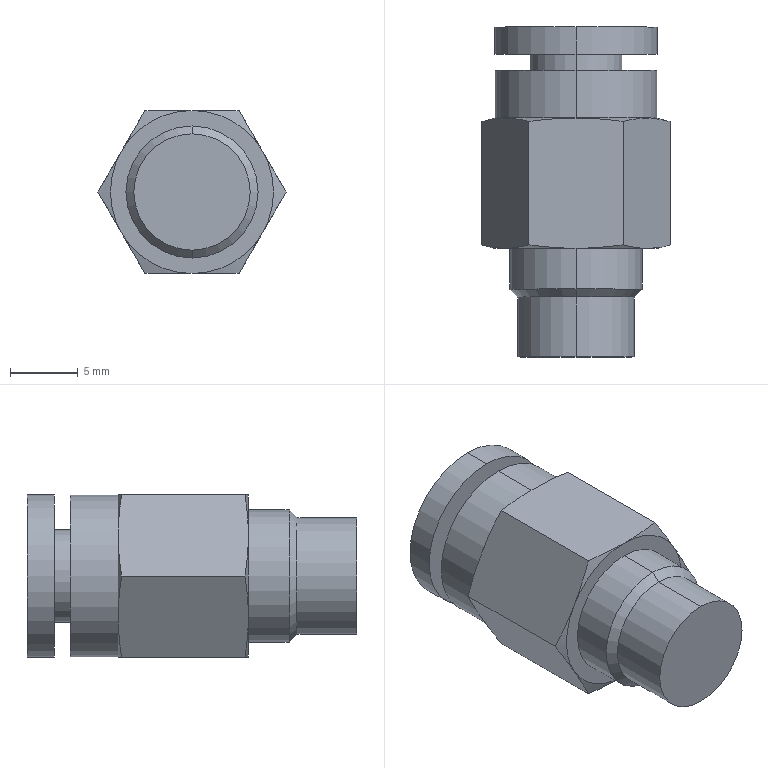Part | STEP file | KQG2H06-01S | 1 solid | 34 faces | box 13.856 x 24.3 x 12 mm | volume 1839 mm3 | cylinder 12 | plane 12 | cone 10 | commonest cylinder face diameters 6 x2 6.8 x2 8.566 x2 9.728 x2 11.9 x2 12 x2
STEP:
#1=CARTESIAN_POINT('',(0.,0.419,4.283));
#2=VERTEX_POINT('',#1);
#3=CARTESIAN_POINT('',(0.,0.419,-4.283));
#4=VERTEX_POINT('',#3);
#5=CARTESIAN_POINT('',(0.,0.419,0.));
#6=DIRECTION('',(0.,-1.,0.));
#7=DIRECTION('',(0.,0.,1.));
#8=AXIS2_PLACEMENT_3D('',#5,#6,#7);
#9=CIRCLE('',#8,4.283);
#10=EDGE_CURVE('',#2,#4,#9,.T.);
#11=ORIENTED_EDGE('',*,*,#10,.F.);
#12=CARTESIAN_POINT('',(0.,1.,4.864));
#13=VERTEX_POINT('',#12);
#14=CARTESIAN_POINT('',(0.,1.,4.864));
#15=DIRECTION('',(0.,0.7071,0.7071));
#16=VECTOR('',#15,1000.);
#17=LINE('',#14,#16);
#18=EDGE_CURVE('',#2,#13,#17,.T.);
#19=ORIENTED_EDGE('',*,*,#18,.T.);
#20=CARTESIAN_POINT('',(0.,1.,-4.864));
#21=VERTEX_POINT('',#20);
#22=CARTESIAN_POINT('',(0.,1.,0.));
#23=DIRECTION('',(0.,-1.,0.));
#24=DIRECTION('',(0.,0.,1.));
#25=AXIS2_PLACEMENT_3D('',#22,#23,#24);
#26=CIRCLE('',#25,4.864);
#27=EDGE_CURVE('',#13,#21,#26,.T.);
#28=ORIENTED_EDGE('',*,*,#27,.T.);
#29=CARTESIAN_POINT('',(0.,1.,-4.864));
#30=DIRECTION('',(0.,0.7071,-0.7071));
#31=VECTOR('',#30,1000.);
#32=LINE('',#29,#31);
#33=EDGE_CURVE('',#4,#21,#32,.T.);
#34=ORIENTED_EDGE('',*,*,#33,.F.);
#35=EDGE_LOOP('',(#11,#19,#28,#34));
#36=FACE_OUTER_BOUND('',#35,.T.);
#37=CARTESIAN_POINT('',(0.,1.,0.));
#38=DIRECTION('',(0.,1.,0.));
#39=DIRECTION('',(0.,0.,-1.));
#40=AXIS2_PLACEMENT_3D('',#37,#38,#39);
#41=CONICAL_SURFACE('',#40,4.864,0.7854);
#42=ADVANCED_FACE('',(#36),#41,.T.);
#43=ORIENTED_EDGE('',*,*,#10,.T.);
#44=CARTESIAN_POINT('',(0.,-4.,-4.283));
#45=VERTEX_POINT('',#44);
#46=CARTESIAN_POINT('',(0.,-5.2,-4.283));
#47=DIRECTION('',(0.,-1.,0.));
#48=VECTOR('',#47,1000.);
#49=LINE('',#46,#48);
#50=EDGE_CURVE('',#4,#45,#49,.T.);
#51=ORIENTED_EDGE('',*,*,#50,.T.);
#52=CARTESIAN_POINT('',(0.,-4.,4.283));
#53=VERTEX_POINT('',#52);
#54=CARTESIAN_POINT('',(0.,-4.,0.));
#55=DIRECTION('',(0.,1.,0.));
#56=DIRECTION('',(0.,0.,1.));
#57=AXIS2_PLACEMENT_3D('',#54,#55,#56);
#58=CIRCLE('',#57,4.283);
#59=EDGE_CURVE('',#45,#53,#58,.T.);
#60=ORIENTED_EDGE('',*,*,#59,.T.);
#61=CARTESIAN_POINT('',(0.,-5.2,4.283));
#62=DIRECTION('',(0.,-1.,0.));
#63=VECTOR('',#62,1000.);
#64=LINE('',#61,#63);
#65=EDGE_CURVE('',#2,#53,#64,.T.);
#66=ORIENTED_EDGE('',*,*,#65,.F.);
#67=EDGE_LOOP('',(#43,#51,#60,#66));
#68=FACE_OUTER_BOUND('',#67,.T.);
#69=CARTESIAN_POINT('',(0.,-5.2,0.));
#70=DIRECTION('',(0.,-1.,0.));
#71=DIRECTION('',(0.,0.,1.));
#72=AXIS2_PLACEMENT_3D('',#69,#70,#71);
#73=CYLINDRICAL_SURFACE('',#72,4.283);
#74=ADVANCED_FACE('',(#68),#73,.T.);
#75=CARTESIAN_POINT('',(0.,1.,0.));
#76=DIRECTION('',(0.,-1.,0.));
#77=DIRECTION('',(0.,0.,1.));
#78=AXIS2_PLACEMENT_3D('',#75,#76,#77);
#79=CIRCLE('',#78,4.864);
#80=EDGE_CURVE('',#21,#13,#79,.T.);
#81=ORIENTED_EDGE('',*,*,#80,.F.);
#82=CARTESIAN_POINT('',(0.,4.,-4.864));
#83=VERTEX_POINT('',#82);
#84=CARTESIAN_POINT('',(0.,20.3,-4.864));
#85=DIRECTION('',(0.,1.,0.));
#86=VECTOR('',#85,1000.);
#87=LINE('',#84,#86);
#88=EDGE_CURVE('',#21,#83,#87,.T.);
#89=ORIENTED_EDGE('',*,*,#88,.T.);
#90=CARTESIAN_POINT('',(0.,4.,4.864));
#91=VERTEX_POINT('',#90);
#92=CARTESIAN_POINT('',(0.,4.,0.));
#93=DIRECTION('',(0.,1.,0.));
#94=DIRECTION('',(0.,0.,1.));
#95=AXIS2_PLACEMENT_3D('',#92,#93,#94);
#96=CIRCLE('',#95,4.864);
#97=EDGE_CURVE('',#91,#83,#96,.T.);
#98=ORIENTED_EDGE('',*,*,#97,.F.);
#99=CARTESIAN_POINT('',(0.,20.3,4.864));
#100=DIRECTION('',(0.,1.,0.));
#101=VECTOR('',#100,1000.);
#102=LINE('',#99,#101);
#103=EDGE_CURVE('',#13,#91,#102,.T.);
#104=ORIENTED_EDGE('',*,*,#103,.F.);
#105=EDGE_LOOP('',(#81,#89,#98,#104));
#106=FACE_OUTER_BOUND('',#105,.T.);
#107=CARTESIAN_POINT('',(0.,20.3,0.));
#108=DIRECTION('',(0.,1.,0.));
#109=DIRECTION('',(0.,0.,1.));
#110=AXIS2_PLACEMENT_3D('',#107,#108,#109);
#111=CYLINDRICAL_SURFACE('',#110,4.864);
#112=ADVANCED_FACE('',(#106),#111,.T.);
#113=CARTESIAN_POINT('',(0.,1.5,-3.));
#114=VERTEX_POINT('',#113);
#115=CARTESIAN_POINT('',(0.,1.5,3.));
#116=VERTEX_POINT('',#115);
#117=CARTESIAN_POINT('',(0.,1.5,0.));
#118=DIRECTION('',(0.,1.,0.));
#119=DIRECTION('',(0.,0.,1.));
#120=AXIS2_PLACEMENT_3D('',#117,#118,#119);
#121=CIRCLE('',#120,3.);
#122=EDGE_CURVE('',#114,#116,#121,.T.);
#123=ORIENTED_EDGE('',*,*,#122,.F.);
#124=CARTESIAN_POINT('',(0.,20.3,-3.));
#125=VERTEX_POINT('',#124);
#126=CARTESIAN_POINT('',(0.,20.3,-3.));
#127=DIRECTION('',(0.,1.,0.));
#128=VECTOR('',#127,1000.);
#129=LINE('',#126,#128);
#130=EDGE_CURVE('',#114,#125,#129,.T.);
#131=ORIENTED_EDGE('',*,*,#130,.T.);
#132=CARTESIAN_POINT('',(0.,20.3,3.));
#133=VERTEX_POINT('',#132);
#134=CARTESIAN_POINT('',(0.,20.3,0.));
#135=DIRECTION('',(0.,1.,0.));
#136=DIRECTION('',(0.,0.,1.));
#137=AXIS2_PLACEMENT_3D('',#134,#135,#136);
#138=CIRCLE('',#137,3.);
#139=EDGE_CURVE('',#125,#133,#138,.T.);
#140=ORIENTED_EDGE('',*,*,#139,.T.);
#141=CARTESIAN_POINT('',(0.,20.3,3.));
#142=DIRECTION('',(0.,1.,0.));
#143=VECTOR('',#142,1000.);
#144=LINE('',#141,#143);
#145=EDGE_CURVE('',#116,#133,#144,.T.);
#146=ORIENTED_EDGE('',*,*,#145,.F.);
#147=EDGE_LOOP('',(#123,#131,#140,#146));
#148=FACE_OUTER_BOUND('',#147,.T.);
#149=CARTESIAN_POINT('',(0.,20.3,0.));
#150=DIRECTION('',(0.,1.,0.));
#151=DIRECTION('',(0.,0.,1.));
#152=AXIS2_PLACEMENT_3D('',#149,#150,#151);
#153=CYLINDRICAL_SURFACE('',#152,3.);
#154=ADVANCED_FACE('',(#148),#153,.F.);
#155=CARTESIAN_POINT('',(0.,18.3,6.));
#156=VERTEX_POINT('',#155);
#157=CARTESIAN_POINT('',(0.,18.3,-6.));
#158=VERTEX_POINT('',#157);
#159=CARTESIAN_POINT('',(0.,18.3,0.));
#160=DIRECTION('',(0.,1.,0.));
#161=DIRECTION('',(0.,0.,1.));
#162=AXIS2_PLACEMENT_3D('',#159,#160,#161);
#163=CIRCLE('',#162,6.);
#164=EDGE_CURVE('',#156,#158,#163,.T.);
#165=ORIENTED_EDGE('',*,*,#164,.T.);
#166=CARTESIAN_POINT('',(0.,20.3,-6.));
#167=VERTEX_POINT('',#166);
#168=CARTESIAN_POINT('',(0.,20.3,-6.));
#169=DIRECTION('',(0.,1.,0.));
#170=VECTOR('',#169,1000.);
#171=LINE('',#168,#170);
#172=EDGE_CURVE('',#158,#167,#171,.T.);
#173=ORIENTED_EDGE('',*,*,#172,.T.);
#174=CARTESIAN_POINT('',(0.,20.3,6.));
#175=VERTEX_POINT('',#174);
#176=CARTESIAN_POINT('',(0.,20.3,0.));
#177=DIRECTION('',(0.,1.,0.));
#178=DIRECTION('',(0.,0.,1.));
#179=AXIS2_PLACEMENT_3D('',#176,#177,#178);
#180=CIRCLE('',#179,6.);
#181=EDGE_CURVE('',#175,#167,#180,.T.);
#182=ORIENTED_EDGE('',*,*,#181,.F.);
#183=CARTESIAN_POINT('',(0.,20.3,6.));
#184=DIRECTION('',(0.,1.,0.));
#185=VECTOR('',#184,1000.);
#186=LINE('',#183,#185);
#187=EDGE_CURVE('',#156,#175,#186,.T.);
#188=ORIENTED_EDGE('',*,*,#187,.F.);
#189=EDGE_LOOP('',(#165,#173,#182,#188));
#190=FACE_OUTER_BOUND('',#189,.T.);
#191=CARTESIAN_POINT('',(0.,20.3,0.));
#192=DIRECTION('',(0.,1.,0.));
#193=DIRECTION('',(0.,0.,1.));
#194=AXIS2_PLACEMENT_3D('',#191,#192,#193);
#195=CYLINDRICAL_SURFACE('',#194,6.);
#196=ADVANCED_FACE('',(#190),#195,.T.);
#197=CARTESIAN_POINT('',(0.,17.1,3.4));
#198=VERTEX_POINT('',#197);
#199=CARTESIAN_POINT('',(0.,17.1,-3.4));
#200=VERTEX_POINT('',#199);
#201=CARTESIAN_POINT('',(0.,17.1,0.));
#202=DIRECTION('',(0.,1.,0.));
#203=DIRECTION('',(0.,0.,1.));
#204=AXIS2_PLACEMENT_3D('',#201,#202,#203);
#205=CIRCLE('',#204,3.4);
#206=EDGE_CURVE('',#198,#200,#205,.T.);
#207=ORIENTED_EDGE('',*,*,#206,.T.);
#208=CARTESIAN_POINT('',(0.,18.3,-3.4));
#209=VERTEX_POINT('',#208);
#210=CARTESIAN_POINT('',(0.,20.3,-3.4));
#211=DIRECTION('',(0.,1.,0.));
#212=VECTOR('',#211,1000.);
#213=LINE('',#210,#212);
#214=EDGE_CURVE('',#200,#209,#213,.T.);
#215=ORIENTED_EDGE('',*,*,#214,.T.);
#216=CARTESIAN_POINT('',(0.,18.3,3.4));
#217=VERTEX_POINT('',#216);
#218=CARTESIAN_POINT('',(0.,18.3,0.));
#219=DIRECTION('',(0.,1.,0.));
#220=DIRECTION('',(0.,0.,1.));
#221=AXIS2_PLACEMENT_3D('',#218,#219,#220);
#222=CIRCLE('',#221,3.4);
#223=EDGE_CURVE('',#217,#209,#222,.T.);
#224=ORIENTED_EDGE('',*,*,#223,.F.);
#225=CARTESIAN_POINT('',(0.,20.3,3.4));
#226=DIRECTION('',(0.,1.,0.));
#227=VECTOR('',#226,1000.);
#228=LINE('',#225,#227);
#229=EDGE_CURVE('',#198,#217,#228,.T.);
#230=ORIENTED_EDGE('',*,*,#229,.F.);
#231=EDGE_LOOP('',(#207,#215,#224,#230));
#232=FACE_OUTER_BOUND('',#231,.T.);
#233=CARTESIAN_POINT('',(0.,20.3,0.));
#234=DIRECTION('',(0.,1.,0.));
#235=DIRECTION('',(0.,0.,1.));
#236=AXIS2_PLACEMENT_3D('',#233,#234,#235);
#237=CYLINDRICAL_SURFACE('',#236,3.4);
#238=ADVANCED_FACE('',(#232),#237,.T.);
#239=CARTESIAN_POINT('',(0.,13.6,5.95));
#240=VERTEX_POINT('',#239);
#241=CARTESIAN_POINT('',(0.,13.6,-5.95));
#242=VERTEX_POINT('',#241);
#243=CARTESIAN_POINT('',(0.,13.6,0.));
#244=DIRECTION('',(0.,1.,0.));
#245=DIRECTION('',(0.,0.,1.));
#246=AXIS2_PLACEMENT_3D('',#243,#244,#245);
#247=CIRCLE('',#246,5.95);
#248=EDGE_CURVE('',#240,#242,#247,.T.);
#249=ORIENTED_EDGE('',*,*,#248,.T.);
#250=CARTESIAN_POINT('',(0.,17.1,-5.95));
#251=VERTEX_POINT('',#250);
#252=CARTESIAN_POINT('',(0.,20.3,-5.95));
#253=DIRECTION('',(0.,1.,0.));
#254=VECTOR('',#253,1000.);
#255=LINE('',#252,#254);
#256=EDGE_CURVE('',#242,#251,#255,.T.);
#257=ORIENTED_EDGE('',*,*,#256,.T.);
#258=CARTESIAN_POINT('',(0.,17.1,5.95));
#259=VERTEX_POINT('',#258);
#260=CARTESIAN_POINT('',(0.,17.1,0.));
#261=DIRECTION('',(0.,1.,0.));
#262=DIRECTION('',(0.,0.,1.));
#263=AXIS2_PLACEMENT_3D('',#260,#261,#262);
#264=CIRCLE('',#263,5.95);
#265=EDGE_CURVE('',#259,#251,#264,.T.);
#266=ORIENTED_EDGE('',*,*,#265,.F.);
#267=CARTESIAN_POINT('',(0.,20.3,5.95));
#268=DIRECTION('',(0.,1.,0.));
#269=VECTOR('',#268,1000.);
#270=LINE('',#267,#269);
#271=EDGE_CURVE('',#240,#259,#270,.T.);
#272=ORIENTED_EDGE('',*,*,#271,.F.);
#273=EDGE_LOOP('',(#249,#257,#266,#272));
#274=FACE_OUTER_BOUND('',#273,.T.);
#275=CARTESIAN_POINT('',(0.,20.3,0.));
#276=DIRECTION('',(0.,1.,0.));
#277=DIRECTION('',(0.,0.,1.));
#278=AXIS2_PLACEMENT_3D('',#275,#276,#277);
#279=CYLINDRICAL_SURFACE('',#278,5.95);
#280=ADVANCED_FACE('',(#274),#279,.T.);
#281=ORIENTED_EDGE('',*,*,#248,.F.);
#282=CARTESIAN_POINT('',(0.,13.587,6.));
#283=VERTEX_POINT('',#282);
#284=CARTESIAN_POINT('',(0.,12.622,9.6));
#285=DIRECTION('',(0.,-0.2588,0.9659));
#286=VECTOR('',#285,1000.);
#287=LINE('',#284,#286);
#288=EDGE_CURVE('',#240,#283,#287,.T.);
#289=ORIENTED_EDGE('',*,*,#288,.T.);
#290=CARTESIAN_POINT('',(3.464,13.338,6.));
#291=VERTEX_POINT('',#290);
#292=CARTESIAN_POINT('',(3.464,13.338,6.));
#293=CARTESIAN_POINT('',(2.318,13.491,6.));
#294=CARTESIAN_POINT('',(1.165,13.587,6.));
#295=CARTESIAN_POINT('',(0.,13.587,6.));
#296=B_SPLINE_CURVE_WITH_KNOTS('',3,(#292,#293,#294,#295),.UNSPECIFIED.,.F.,.F.,(4,4),(0.007115,0.01058),.UNSPECIFIED.);
#297=EDGE_CURVE('',#291,#283,#296,.T.);
#298=ORIENTED_EDGE('',*,*,#297,.F.);
#299=CARTESIAN_POINT('',(6.928,13.338,0.));
#300=VERTEX_POINT('',#299);
#301=CARTESIAN_POINT('',(6.928,13.338,0.));
#302=CARTESIAN_POINT('',(6.351,13.493,1.));
#303=CARTESIAN_POINT('',(5.196,13.681,3.));
#304=CARTESIAN_POINT('',(4.041,13.493,5.));
#305=CARTESIAN_POINT('',(3.464,13.338,6.));
#306=B_SPLINE_CURVE_WITH_KNOTS('',3,(#301,#302,#303,#304,#305),.UNSPECIFIED.,.F.,.F.,(4,1,4),(0.000000231,0.003464,0.006928),.UNSPECIFIED.);
#307=EDGE_CURVE('',#300,#291,#306,.T.);
#308=ORIENTED_EDGE('',*,*,#307,.F.);
#309=CARTESIAN_POINT('',(3.464,13.338,-6.));
#310=VERTEX_POINT('',#309);
#311=CARTESIAN_POINT('',(3.464,13.338,-6.));
#312=CARTESIAN_POINT('',(4.041,13.493,-5.));
#313=CARTESIAN_POINT('',(5.196,13.681,-3.));
#314=CARTESIAN_POINT('',(6.351,13.493,-1.));
#315=CARTESIAN_POINT('',(6.928,13.338,0.));
#316=B_SPLINE_CURVE_WITH_KNOTS('',3,(#311,#312,#313,#314,#315),.UNSPECIFIED.,.F.,.F.,(4,1,4),(0.000000231,0.003464,0.006928),.UNSPECIFIED.);
#317=EDGE_CURVE('',#310,#300,#316,.T.);
#318=ORIENTED_EDGE('',*,*,#317,.F.);
#319=CARTESIAN_POINT('',(0.,13.587,-6.));
#320=VERTEX_POINT('',#319);
#321=CARTESIAN_POINT('',(0.,13.587,-6.));
#322=CARTESIAN_POINT('',(0.5747,13.587,-6.));
#323=CARTESIAN_POINT('',(1.152,13.564,-6.));
#324=CARTESIAN_POINT('',(2.313,13.478,-6.));
#325=CARTESIAN_POINT('',(2.89,13.415,-6.));
#326=CARTESIAN_POINT('',(3.464,13.338,-6.));
#327=B_SPLINE_CURVE_WITH_KNOTS('',3,(#321,#322,#323,#324,#325,#326),.UNSPECIFIED.,.F.,.F.,(4,2,4),(0.01058,0.01229,0.014),.UNSPECIFIED.);
#328=EDGE_CURVE('',#320,#310,#327,.T.);
#329=ORIENTED_EDGE('',*,*,#328,.F.);
#330=CARTESIAN_POINT('',(0.,12.622,-9.6));
#331=DIRECTION('',(0.,-0.2588,-0.9659));
#332=VECTOR('',#331,1000.);
#333=LINE('',#330,#332);
#334=EDGE_CURVE('',#242,#320,#333,.T.);
#335=ORIENTED_EDGE('',*,*,#334,.F.);
#336=EDGE_LOOP('',(#281,#289,#298,#308,#318,#329,#335));
#337=FACE_OUTER_BOUND('',#336,.T.);
#338=CARTESIAN_POINT('',(0.,12.622,0.));
#339=DIRECTION('',(0.,-1.,0.));
#340=DIRECTION('',(0.,0.,-1.));
#341=AXIS2_PLACEMENT_3D('',#338,#339,#340);
#342=CONICAL_SURFACE('',#341,9.6,1.309);
#343=ADVANCED_FACE('',(#337),#342,.T.);
#344=ORIENTED_EDGE('',*,*,#288,.F.);
#345=CARTESIAN_POINT('',(0.,13.6,0.));
#346=DIRECTION('',(0.,1.,0.));
#347=DIRECTION('',(0.,0.,1.));
#348=AXIS2_PLACEMENT_3D('',#345,#346,#347);
#349=CIRCLE('',#348,5.95);
#350=EDGE_CURVE('',#242,#240,#349,.T.);
#351=ORIENTED_EDGE('',*,*,#350,.F.);
#352=ORIENTED_EDGE('',*,*,#334,.T.);
#353=CARTESIAN_POINT('',(-3.464,13.338,-6.));
#354=VERTEX_POINT('',#353);
#355=CARTESIAN_POINT('',(-3.464,13.338,-6.));
#356=CARTESIAN_POINT('',(-2.318,13.491,-6.));
#357=CARTESIAN_POINT('',(-1.165,13.587,-6.));
#358=CARTESIAN_POINT('',(0.,13.587,-6.));
#359=B_SPLINE_CURVE_WITH_KNOTS('',3,(#355,#356,#357,#358),.UNSPECIFIED.,.F.,.F.,(4,4),(0.007115,0.01058),.UNSPECIFIED.);
#360=EDGE_CURVE('',#354,#320,#359,.T.);
#361=ORIENTED_EDGE('',*,*,#360,.F.);
#362=CARTESIAN_POINT('',(-6.928,13.338,0.));
#363=VERTEX_POINT('',#362);
#364=CARTESIAN_POINT('',(-6.928,13.338,0.));
#365=CARTESIAN_POINT('',(-6.351,13.493,-1.));
#366=CARTESIAN_POINT('',(-5.196,13.681,-3.));
#367=CARTESIAN_POINT('',(-4.041,13.493,-5.));
#368=CARTESIAN_POINT('',(-3.464,13.338,-6.));
#369=B_SPLINE_CURVE_WITH_KNOTS('',3,(#364,#365,#366,#367,#368),.UNSPECIFIED.,.F.,.F.,(4,1,4),(0.000000231,0.003464,0.006928),.UNSPECIFIED.);
#370=EDGE_CURVE('',#363,#354,#369,.T.);
#371=ORIENTED_EDGE('',*,*,#370,.F.);
#372=CARTESIAN_POINT('',(-3.464,13.338,6.));
#373=VERTEX_POINT('',#372);
#374=CARTESIAN_POINT('',(-3.464,13.338,6.));
#375=CARTESIAN_POINT('',(-4.041,13.493,5.));
#376=CARTESIAN_POINT('',(-5.196,13.681,3.));
#377=CARTESIAN_POINT('',(-6.351,13.493,1.));
#378=CARTESIAN_POINT('',(-6.928,13.338,0.));
#379=B_SPLINE_CURVE_WITH_KNOTS('',3,(#374,#375,#376,#377,#378),.UNSPECIFIED.,.F.,.F.,(4,1,4),(0.000000231,0.003464,0.006928),.UNSPECIFIED.);
#380=EDGE_CURVE('',#373,#363,#379,.T.);
#381=ORIENTED_EDGE('',*,*,#380,.F.);
#382=CARTESIAN_POINT('',(0.,13.587,6.));
#383=CARTESIAN_POINT('',(-0.5747,13.587,6.));
#384=CARTESIAN_POINT('',(-1.152,13.564,6.));
#385=CARTESIAN_POINT('',(-2.313,13.478,6.));
#386=CARTESIAN_POINT('',(-2.89,13.415,6.));
#387=CARTESIAN_POINT('',(-3.464,13.338,6.));
#388=B_SPLINE_CURVE_WITH_KNOTS('',3,(#382,#383,#384,#385,#386,#387),.UNSPECIFIED.,.F.,.F.,(4,2,4),(0.01058,0.01229,0.014),.UNSPECIFIED.);
#389=EDGE_CURVE('',#283,#373,#388,.T.);
#390=ORIENTED_EDGE('',*,*,#389,.F.);
#391=EDGE_LOOP('',(#344,#351,#352,#361,#371,#381,#390));
#392=FACE_OUTER_BOUND('',#391,.T.);
#393=CARTESIAN_POINT('',(0.,12.622,0.));
#394=DIRECTION('',(0.,-1.,0.));
#395=DIRECTION('',(0.,0.,-1.));
#396=AXIS2_PLACEMENT_3D('',#393,#394,#395);
#397=CONICAL_SURFACE('',#396,9.6,1.309);
#398=ADVANCED_FACE('',(#392),#397,.T.);
#399=ORIENTED_EDGE('',*,*,#256,.F.);
#400=ORIENTED_EDGE('',*,*,#350,.T.);
#401=ORIENTED_EDGE('',*,*,#271,.T.);
#402=CARTESIAN_POINT('',(0.,17.1,0.));
#403=DIRECTION('',(0.,1.,0.));
#404=DIRECTION('',(0.,0.,1.));
#405=AXIS2_PLACEMENT_3D('',#402,#403,#404);
#406=CIRCLE('',#405,5.95);
#407=EDGE_CURVE('',#251,#259,#406,.T.);
#408=ORIENTED_EDGE('',*,*,#407,.F.);
#409=EDGE_LOOP('',(#399,#400,#401,#408));
#410=FACE_OUTER_BOUND('',#409,.T.);
#411=CARTESIAN_POINT('',(0.,20.3,0.));
#412=DIRECTION('',(0.,1.,0.));
#413=DIRECTION('',(0.,0.,1.));
#414=AXIS2_PLACEMENT_3D('',#411,#412,#413);
#415=CYLINDRICAL_SURFACE('',#414,5.95);
#416=ADVANCED_FACE('',(#410),#415,.T.);
#417=ORIENTED_EDGE('',*,*,#206,.F.);
#418=CARTESIAN_POINT('',(0.,17.1,0.));
#419=DIRECTION('',(0.,1.,0.));
#420=DIRECTION('',(0.,0.,1.));
#421=AXIS2_PLACEMENT_3D('',#418,#419,#420);
#422=CIRCLE('',#421,3.4);
#423=EDGE_CURVE('',#200,#198,#422,.T.);
#424=ORIENTED_EDGE('',*,*,#423,.F.);
#425=EDGE_LOOP('',(#417,#424));
#426=FACE_BOUND('',#425,.T.);
#427=ORIENTED_EDGE('',*,*,#265,.T.);
#428=ORIENTED_EDGE('',*,*,#407,.T.);
#429=EDGE_LOOP('',(#427,#428));
#430=FACE_OUTER_BOUND('',#429,.T.);
#431=CARTESIAN_POINT('',(-5.95,17.1,0.));
#432=DIRECTION('',(0.,-1.,0.));
#433=DIRECTION('',(0.,0.,-1.));
#434=AXIS2_PLACEMENT_3D('',#431,#432,#433);
#435=PLANE('',#434);
#436=ADVANCED_FACE('',(#426,#430),#435,.F.);
#437=ORIENTED_EDGE('',*,*,#214,.F.);
#438=ORIENTED_EDGE('',*,*,#423,.T.);
#439=ORIENTED_EDGE('',*,*,#229,.T.);
#440=CARTESIAN_POINT('',(0.,18.3,0.));
#441=DIRECTION('',(0.,1.,0.));
#442=DIRECTION('',(0.,0.,1.));
#443=AXIS2_PLACEMENT_3D('',#440,#441,#442);
#444=CIRCLE('',#443,3.4);
#445=EDGE_CURVE('',#209,#217,#444,.T.);
#446=ORIENTED_EDGE('',*,*,#445,.F.);
#447=EDGE_LOOP('',(#437,#438,#439,#446));
#448=FACE_OUTER_BOUND('',#447,.T.);
#449=CARTESIAN_POINT('',(0.,20.3,0.));
#450=DIRECTION('',(0.,1.,0.));
#451=DIRECTION('',(0.,0.,1.));
#452=AXIS2_PLACEMENT_3D('',#449,#450,#451);
#453=CYLINDRICAL_SURFACE('',#452,3.4);
#454=ADVANCED_FACE('',(#448),#453,.T.);
#455=ORIENTED_EDGE('',*,*,#164,.F.);
#456=CARTESIAN_POINT('',(0.,18.3,0.));
#457=DIRECTION('',(0.,1.,0.));
#458=DIRECTION('',(0.,0.,1.));
#459=AXIS2_PLACEMENT_3D('',#456,#457,#458);
#460=CIRCLE('',#459,6.);
#461=EDGE_CURVE('',#158,#156,#460,.T.);
#462=ORIENTED_EDGE('',*,*,#461,.F.);
#463=EDGE_LOOP('',(#455,#462));
#464=FACE_OUTER_BOUND('',#463,.T.);
#465=ORIENTED_EDGE('',*,*,#223,.T.);
#466=ORIENTED_EDGE('',*,*,#445,.T.);
#467=EDGE_LOOP('',(#465,#466));
#468=FACE_BOUND('',#467,.T.);
#469=CARTESIAN_POINT('',(-3.4,18.3,0.));
#470=DIRECTION('',(0.,1.,0.));
#471=DIRECTION('',(0.,0.,1.));
#472=AXIS2_PLACEMENT_3D('',#469,#470,#471);
#473=PLANE('',#472);
#474=ADVANCED_FACE('',(#464,#468),#473,.F.);
#475=ORIENTED_EDGE('',*,*,#172,.F.);
#476=ORIENTED_EDGE('',*,*,#461,.T.);
#477=ORIENTED_EDGE('',*,*,#187,.T.);
#478=CARTESIAN_POINT('',(0.,20.3,0.));
#479=DIRECTION('',(0.,1.,0.));
#480=DIRECTION('',(0.,0.,1.));
#481=AXIS2_PLACEMENT_3D('',#478,#479,#480);
#482=CIRCLE('',#481,6.);
#483=EDGE_CURVE('',#167,#175,#482,.T.);
#484=ORIENTED_EDGE('',*,*,#483,.F.);
#485=EDGE_LOOP('',(#475,#476,#477,#484));
#486=FACE_OUTER_BOUND('',#485,.T.);
#487=CARTESIAN_POINT('',(0.,20.3,0.));
#488=DIRECTION('',(0.,1.,0.));
#489=DIRECTION('',(0.,0.,1.));
#490=AXIS2_PLACEMENT_3D('',#487,#488,#489);
#491=CYLINDRICAL_SURFACE('',#490,6.);
#492=ADVANCED_FACE('',(#486),#491,.T.);
#493=CARTESIAN_POINT('',(0.,20.3,0.));
#494=DIRECTION('',(0.,1.,0.));
#495=DIRECTION('',(0.,0.,1.));
#496=AXIS2_PLACEMENT_3D('',#493,#494,#495);
#497=CIRCLE('',#496,3.);
#498=EDGE_CURVE('',#133,#125,#497,.T.);
#499=ORIENTED_EDGE('',*,*,#498,.F.);
#500=ORIENTED_EDGE('',*,*,#139,.F.);
#501=EDGE_LOOP('',(#499,#500));
#502=FACE_BOUND('',#501,.T.);
#503=ORIENTED_EDGE('',*,*,#181,.T.);
#504=ORIENTED_EDGE('',*,*,#483,.T.);
#505=EDGE_LOOP('',(#503,#504));
#506=FACE_OUTER_BOUND('',#505,.T.);
#507=CARTESIAN_POINT('',(-6.,20.3,0.));
#508=DIRECTION('',(0.,-1.,0.));
#509=DIRECTION('',(0.,0.,-1.));
#510=AXIS2_PLACEMENT_3D('',#507,#508,#509);
#511=PLANE('',#510);
#512=ADVANCED_FACE('',(#502,#506),#511,.F.);
#513=ORIENTED_EDGE('',*,*,#130,.F.);
#514=CARTESIAN_POINT('',(0.,1.5,0.));
#515=DIRECTION('',(0.,1.,0.));
#516=DIRECTION('',(0.,0.,1.));
#517=AXIS2_PLACEMENT_3D('',#514,#515,#516);
#518=CIRCLE('',#517,3.);
#519=EDGE_CURVE('',#116,#114,#518,.T.);
#520=ORIENTED_EDGE('',*,*,#519,.F.);
#521=ORIENTED_EDGE('',*,*,#145,.T.);
#522=ORIENTED_EDGE('',*,*,#498,.T.);
#523=EDGE_LOOP('',(#513,#520,#521,#522));
#524=FACE_OUTER_BOUND('',#523,.T.);
#525=CARTESIAN_POINT('',(0.,20.3,0.));
#526=DIRECTION('',(0.,1.,0.));
#527=DIRECTION('',(0.,0.,1.));
#528=AXIS2_PLACEMENT_3D('',#525,#526,#527);
#529=CYLINDRICAL_SURFACE('',#528,3.);
#530=ADVANCED_FACE('',(#524),#529,.F.);
#531=ORIENTED_EDGE('',*,*,#519,.T.);
#532=ORIENTED_EDGE('',*,*,#122,.T.);
#533=EDGE_LOOP('',(#531,#532));
#534=FACE_OUTER_BOUND('',#533,.T.);
#535=CARTESIAN_POINT('',(-3.,1.5,0.));
#536=DIRECTION('',(0.,-1.,0.));
#537=DIRECTION('',(0.,0.,-1.));
#538=AXIS2_PLACEMENT_3D('',#535,#536,#537);
#539=PLANE('',#538);
#540=ADVANCED_FACE('',(#534),#539,.F.);
#541=CARTESIAN_POINT('',(6.928,4.249,0.));
#542=VERTEX_POINT('',#541);
#543=CARTESIAN_POINT('',(5.196,4.,-3.));
#544=VERTEX_POINT('',#543);
#545=CARTESIAN_POINT('',(6.928,4.249,0.));
#546=CARTESIAN_POINT('',(6.351,4.094,-1.));
#547=CARTESIAN_POINT('',(5.774,4.,-2.));
#548=CARTESIAN_POINT('',(5.196,4.,-3.));
#549=B_SPLINE_CURVE_WITH_KNOTS('',3,(#545,#546,#547,#548),.UNSPECIFIED.,.F.,.F.,(4,4),(0.000000231,0.003464),.UNSPECIFIED.);
#550=EDGE_CURVE('',#542,#544,#549,.T.);
#551=ORIENTED_EDGE('',*,*,#550,.T.);
#552=CARTESIAN_POINT('',(3.464,4.249,-6.));
#553=VERTEX_POINT('',#552);
#554=CARTESIAN_POINT('',(5.196,4.,-3.));
#555=CARTESIAN_POINT('',(4.619,4.,-4.));
#556=CARTESIAN_POINT('',(4.041,4.094,-5.));
#557=CARTESIAN_POINT('',(3.464,4.249,-6.));
#558=B_SPLINE_CURVE_WITH_KNOTS('',3,(#554,#555,#556,#557),.UNSPECIFIED.,.F.,.F.,(4,4),(0.003464,0.006928),.UNSPECIFIED.);
#559=EDGE_CURVE('',#544,#553,#558,.T.);
#560=ORIENTED_EDGE('',*,*,#559,.T.);
#561=CARTESIAN_POINT('',(3.464,13.6,-6.));
#562=DIRECTION('',(0.,-1.,0.));
#563=VECTOR('',#562,1000.);
#564=LINE('',#561,#563);
#565=EDGE_CURVE('',#310,#553,#564,.T.);
#566=ORIENTED_EDGE('',*,*,#565,.F.);
#567=ORIENTED_EDGE('',*,*,#317,.T.);
#568=CARTESIAN_POINT('',(6.928,13.6,0.));
#569=DIRECTION('',(0.,-1.,0.));
#570=VECTOR('',#569,1000.);
#571=LINE('',#568,#570);
#572=EDGE_CURVE('',#300,#542,#571,.T.);
#573=ORIENTED_EDGE('',*,*,#572,.T.);
#574=EDGE_LOOP('',(#551,#560,#566,#567,#573));
#575=FACE_OUTER_BOUND('',#574,.T.);
#576=CARTESIAN_POINT('',(3.464,13.6,-6.));
#577=DIRECTION('',(0.866,0.,-0.5));
#578=DIRECTION('',(-0.5,0.,-0.866));
#579=AXIS2_PLACEMENT_3D('',#576,#577,#578);
#580=PLANE('',#579);
#581=ADVANCED_FACE('',(#575),#580,.T.);
#582=CARTESIAN_POINT('',(0.,4.,-6.));
#583=VERTEX_POINT('',#582);
#584=CARTESIAN_POINT('',(3.464,4.249,-6.));
#585=CARTESIAN_POINT('',(2.318,4.095,-6.));
#586=CARTESIAN_POINT('',(1.165,4.,-6.));
#587=CARTESIAN_POINT('',(0.,4.,-6.));
#588=B_SPLINE_CURVE_WITH_KNOTS('',3,(#584,#585,#586,#587),.UNSPECIFIED.,.F.,.F.,(4,4),(0.007113,0.01058),.UNSPECIFIED.);
#589=EDGE_CURVE('',#553,#583,#588,.T.);
#590=ORIENTED_EDGE('',*,*,#589,.T.);
#591=CARTESIAN_POINT('',(-3.464,4.249,-6.));
#592=VERTEX_POINT('',#591);
#593=CARTESIAN_POINT('',(0.,4.,-6.));
#594=CARTESIAN_POINT('',(-0.5747,4.,-6.));
#595=CARTESIAN_POINT('',(-1.152,4.023,-6.));
#596=CARTESIAN_POINT('',(-2.313,4.109,-6.));
#597=CARTESIAN_POINT('',(-2.89,4.172,-6.));
#598=CARTESIAN_POINT('',(-3.464,4.249,-6.));
#599=B_SPLINE_CURVE_WITH_KNOTS('',3,(#593,#594,#595,#596,#597,#598),.UNSPECIFIED.,.F.,.F.,(4,2,4),(0.01058,0.01229,0.014),.UNSPECIFIED.);
#600=EDGE_CURVE('',#583,#592,#599,.T.);
#601=ORIENTED_EDGE('',*,*,#600,.T.);
#602=CARTESIAN_POINT('',(-3.464,13.6,-6.));
#603=DIRECTION('',(0.,-1.,0.));
#604=VECTOR('',#603,1000.);
#605=LINE('',#602,#604);
#606=EDGE_CURVE('',#354,#592,#605,.T.);
#607=ORIENTED_EDGE('',*,*,#606,.F.);
#608=ORIENTED_EDGE('',*,*,#360,.T.);
#609=ORIENTED_EDGE('',*,*,#328,.T.);
#610=ORIENTED_EDGE('',*,*,#565,.T.);
#611=EDGE_LOOP('',(#590,#601,#607,#608,#609,#610));
#612=FACE_OUTER_BOUND('',#611,.T.);
#613=CARTESIAN_POINT('',(-3.464,13.6,-6.));
#614=DIRECTION('',(0.,0.,-1.));
#615=DIRECTION('',(-1.,0.,0.));
#616=AXIS2_PLACEMENT_3D('',#613,#614,#615);
#617=PLANE('',#616);
#618=ADVANCED_FACE('',(#612),#617,.T.);
#619=CARTESIAN_POINT('',(-5.196,4.,-3.));
#620=VERTEX_POINT('',#619);
#621=CARTESIAN_POINT('',(-3.464,4.249,-6.));
#622=CARTESIAN_POINT('',(-4.041,4.094,-5.));
#623=CARTESIAN_POINT('',(-4.619,4.,-4.));
#624=CARTESIAN_POINT('',(-5.196,4.,-3.));
#625=B_SPLINE_CURVE_WITH_KNOTS('',3,(#621,#622,#623,#624),.UNSPECIFIED.,.F.,.F.,(4,4),(0.000000231,0.003464),.UNSPECIFIED.);
#626=EDGE_CURVE('',#592,#620,#625,.T.);
#627=ORIENTED_EDGE('',*,*,#626,.T.);
#628=CARTESIAN_POINT('',(-6.928,4.249,0.));
#629=VERTEX_POINT('',#628);
#630=CARTESIAN_POINT('',(-5.196,4.,-3.));
#631=CARTESIAN_POINT('',(-5.774,4.,-2.));
#632=CARTESIAN_POINT('',(-6.351,4.094,-1.));
#633=CARTESIAN_POINT('',(-6.928,4.249,0.));
#634=B_SPLINE_CURVE_WITH_KNOTS('',3,(#630,#631,#632,#633),.UNSPECIFIED.,.F.,.F.,(4,4),(0.003464,0.006928),.UNSPECIFIED.);
#635=EDGE_CURVE('',#620,#629,#634,.T.);
#636=ORIENTED_EDGE('',*,*,#635,.T.);
#637=CARTESIAN_POINT('',(-6.928,13.6,0.));
#638=DIRECTION('',(0.,-1.,0.));
#639=VECTOR('',#638,1000.);
#640=LINE('',#637,#639);
#641=EDGE_CURVE('',#363,#629,#640,.T.);
#642=ORIENTED_EDGE('',*,*,#641,.F.);
#643=ORIENTED_EDGE('',*,*,#370,.T.);
#644=ORIENTED_EDGE('',*,*,#606,.T.);
#645=EDGE_LOOP('',(#627,#636,#642,#643,#644));
#646=FACE_OUTER_BOUND('',#645,.T.);
#647=CARTESIAN_POINT('',(-6.928,13.6,0.));
#648=DIRECTION('',(-0.866,0.,-0.5));
#649=DIRECTION('',(-0.5,0.,0.866));
#650=AXIS2_PLACEMENT_3D('',#647,#648,#649);
#651=PLANE('',#650);
#652=ADVANCED_FACE('',(#646),#651,.T.);
#653=CARTESIAN_POINT('',(-5.196,4.,3.));
#654=VERTEX_POINT('',#653);
#655=CARTESIAN_POINT('',(-6.928,4.249,0.));
#656=CARTESIAN_POINT('',(-6.351,4.094,1.));
#657=CARTESIAN_POINT('',(-5.774,4.,2.));
#658=CARTESIAN_POINT('',(-5.196,4.,3.));
#659=B_SPLINE_CURVE_WITH_KNOTS('',3,(#655,#656,#657,#658),.UNSPECIFIED.,.F.,.F.,(4,4),(0.000000231,0.003464),.UNSPECIFIED.);
#660=EDGE_CURVE('',#629,#654,#659,.T.);
#661=ORIENTED_EDGE('',*,*,#660,.T.);
#662=CARTESIAN_POINT('',(-3.464,4.249,6.));
#663=VERTEX_POINT('',#662);
#664=CARTESIAN_POINT('',(-5.196,4.,3.));
#665=CARTESIAN_POINT('',(-4.619,4.,4.));
#666=CARTESIAN_POINT('',(-4.041,4.094,5.));
#667=CARTESIAN_POINT('',(-3.464,4.249,6.));
#668=B_SPLINE_CURVE_WITH_KNOTS('',3,(#664,#665,#666,#667),.UNSPECIFIED.,.F.,.F.,(4,4),(0.003464,0.006928),.UNSPECIFIED.);
#669=EDGE_CURVE('',#654,#663,#668,.T.);
#670=ORIENTED_EDGE('',*,*,#669,.T.);
#671=CARTESIAN_POINT('',(-3.464,13.6,6.));
#672=DIRECTION('',(0.,-1.,0.));
#673=VECTOR('',#672,1000.);
#674=LINE('',#671,#673);
#675=EDGE_CURVE('',#373,#663,#674,.T.);
#676=ORIENTED_EDGE('',*,*,#675,.F.);
#677=ORIENTED_EDGE('',*,*,#380,.T.);
#678=ORIENTED_EDGE('',*,*,#641,.T.);
#679=EDGE_LOOP('',(#661,#670,#676,#677,#678));
#680=FACE_OUTER_BOUND('',#679,.T.);
#681=CARTESIAN_POINT('',(-3.464,13.6,6.));
#682=DIRECTION('',(-0.866,0.,0.5));
#683=DIRECTION('',(0.5,0.,0.866));
#684=AXIS2_PLACEMENT_3D('',#681,#682,#683);
#685=PLANE('',#684);
#686=ADVANCED_FACE('',(#680),#685,.T.);
#687=CARTESIAN_POINT('',(0.,4.,6.));
#688=VERTEX_POINT('',#687);
#689=CARTESIAN_POINT('',(-3.464,4.249,6.));
#690=CARTESIAN_POINT('',(-2.318,4.095,6.));
#691=CARTESIAN_POINT('',(-1.165,4.,6.));
#692=CARTESIAN_POINT('',(0.,4.,6.));
#693=B_SPLINE_CURVE_WITH_KNOTS('',3,(#689,#690,#691,#692),.UNSPECIFIED.,.F.,.F.,(4,4),(0.007113,0.01058),.UNSPECIFIED.);
#694=EDGE_CURVE('',#663,#688,#693,.T.);
#695=ORIENTED_EDGE('',*,*,#694,.T.);
#696=CARTESIAN_POINT('',(3.464,4.249,6.));
#697=VERTEX_POINT('',#696);
#698=CARTESIAN_POINT('',(0.,4.,6.));
#699=CARTESIAN_POINT('',(0.5747,4.,6.));
#700=CARTESIAN_POINT('',(1.152,4.023,6.));
#701=CARTESIAN_POINT('',(2.313,4.109,6.));
#702=CARTESIAN_POINT('',(2.89,4.172,6.));
#703=CARTESIAN_POINT('',(3.464,4.249,6.));
#704=B_SPLINE_CURVE_WITH_KNOTS('',3,(#698,#699,#700,#701,#702,#703),.UNSPECIFIED.,.F.,.F.,(4,2,4),(0.01058,0.01229,0.014),.UNSPECIFIED.);
#705=EDGE_CURVE('',#688,#697,#704,.T.);
#706=ORIENTED_EDGE('',*,*,#705,.T.);
#707=CARTESIAN_POINT('',(3.464,13.6,6.));
#708=DIRECTION('',(0.,-1.,0.));
#709=VECTOR('',#708,1000.);
#710=LINE('',#707,#709);
#711=EDGE_CURVE('',#291,#697,#710,.T.);
#712=ORIENTED_EDGE('',*,*,#711,.F.);
#713=ORIENTED_EDGE('',*,*,#297,.T.);
#714=ORIENTED_EDGE('',*,*,#389,.T.);
#715=ORIENTED_EDGE('',*,*,#675,.T.);
#716=EDGE_LOOP('',(#695,#706,#712,#713,#714,#715));
#717=FACE_OUTER_BOUND('',#716,.T.);
#718=CARTESIAN_POINT('',(3.464,13.6,6.));
#719=DIRECTION('',(0.,0.,1.));
#720=DIRECTION('',(1.,0.,0.));
#721=AXIS2_PLACEMENT_3D('',#718,#719,#720);
#722=PLANE('',#721);
#723=ADVANCED_FACE('',(#717),#722,.T.);
#724=CARTESIAN_POINT('',(5.196,4.,3.));
#725=VERTEX_POINT('',#724);
#726=CARTESIAN_POINT('',(3.464,4.249,6.));
#727=CARTESIAN_POINT('',(4.041,4.094,5.));
#728=CARTESIAN_POINT('',(4.619,4.,4.));
#729=CARTESIAN_POINT('',(5.196,4.,3.));
#730=B_SPLINE_CURVE_WITH_KNOTS('',3,(#726,#727,#728,#729),.UNSPECIFIED.,.F.,.F.,(4,4),(0.000000231,0.003464),.UNSPECIFIED.);
#731=EDGE_CURVE('',#697,#725,#730,.T.);
#732=ORIENTED_EDGE('',*,*,#731,.T.);
#733=CARTESIAN_POINT('',(5.196,4.,3.));
#734=CARTESIAN_POINT('',(5.774,4.,2.));
#735=CARTESIAN_POINT('',(6.351,4.094,1.));
#736=CARTESIAN_POINT('',(6.928,4.249,0.));
#737=B_SPLINE_CURVE_WITH_KNOTS('',3,(#733,#734,#735,#736),.UNSPECIFIED.,.F.,.F.,(4,4),(0.003464,0.006928),.UNSPECIFIED.);
#738=EDGE_CURVE('',#725,#542,#737,.T.);
#739=ORIENTED_EDGE('',*,*,#738,.T.);
#740=ORIENTED_EDGE('',*,*,#572,.F.);
#741=ORIENTED_EDGE('',*,*,#307,.T.);
#742=ORIENTED_EDGE('',*,*,#711,.T.);
#743=EDGE_LOOP('',(#732,#739,#740,#741,#742));
#744=FACE_OUTER_BOUND('',#743,.T.);
#745=CARTESIAN_POINT('',(6.928,13.6,0.));
#746=DIRECTION('',(0.866,0.,0.5));
#747=DIRECTION('',(0.5,0.,-0.866));
#748=AXIS2_PLACEMENT_3D('',#745,#746,#747);
#749=PLANE('',#748);
#750=ADVANCED_FACE('',(#744),#749,.T.);
#751=ORIENTED_EDGE('',*,*,#88,.F.);
#752=ORIENTED_EDGE('',*,*,#27,.F.);
#753=ORIENTED_EDGE('',*,*,#103,.T.);
#754=CARTESIAN_POINT('',(0.,4.,0.));
#755=DIRECTION('',(0.,1.,0.));
#756=DIRECTION('',(0.,0.,1.));
#757=AXIS2_PLACEMENT_3D('',#754,#755,#756);
#758=CIRCLE('',#757,4.864);
#759=EDGE_CURVE('',#83,#91,#758,.T.);
#760=ORIENTED_EDGE('',*,*,#759,.F.);
#761=EDGE_LOOP('',(#751,#752,#753,#760));
#762=FACE_OUTER_BOUND('',#761,.T.);
#763=CARTESIAN_POINT('',(0.,20.3,0.));
#764=DIRECTION('',(0.,1.,0.));
#765=DIRECTION('',(0.,0.,1.));
#766=AXIS2_PLACEMENT_3D('',#763,#764,#765);
#767=CYLINDRICAL_SURFACE('',#766,4.864);
#768=ADVANCED_FACE('',(#762),#767,.T.);
#769=ORIENTED_EDGE('',*,*,#669,.F.);
#770=CARTESIAN_POINT('',(0.,4.,0.));
#771=DIRECTION('',(0.,1.,0.));
#772=DIRECTION('',(0.,0.,1.));
#773=AXIS2_PLACEMENT_3D('',#770,#771,#772);
#774=CIRCLE('',#773,6.);
#775=EDGE_CURVE('',#654,#688,#774,.T.);
#776=ORIENTED_EDGE('',*,*,#775,.T.);
#777=ORIENTED_EDGE('',*,*,#694,.F.);
#778=EDGE_LOOP('',(#769,#776,#777));
#779=FACE_OUTER_BOUND('',#778,.T.);
#780=CARTESIAN_POINT('',(0.,4.,0.));
#781=DIRECTION('',(0.,1.,0.));
#782=DIRECTION('',(0.,0.,1.));
#783=AXIS2_PLACEMENT_3D('',#780,#781,#782);
#784=CONICAL_SURFACE('',#783,6.,1.309);
#785=ADVANCED_FACE('',(#779),#784,.T.);
#786=ORIENTED_EDGE('',*,*,#705,.F.);
#787=CARTESIAN_POINT('',(0.,4.,0.));
#788=DIRECTION('',(0.,1.,0.));
#789=DIRECTION('',(0.,0.,1.));
#790=AXIS2_PLACEMENT_3D('',#787,#788,#789);
#791=CIRCLE('',#790,6.);
#792=EDGE_CURVE('',#688,#725,#791,.T.);
#793=ORIENTED_EDGE('',*,*,#792,.T.);
#794=ORIENTED_EDGE('',*,*,#731,.F.);
#795=EDGE_LOOP('',(#786,#793,#794));
#796=FACE_OUTER_BOUND('',#795,.T.);
#797=CARTESIAN_POINT('',(0.,4.,0.));
#798=DIRECTION('',(0.,1.,0.));
#799=DIRECTION('',(0.,0.,1.));
#800=AXIS2_PLACEMENT_3D('',#797,#798,#799);
#801=CONICAL_SURFACE('',#800,6.,1.309);
#802=ADVANCED_FACE('',(#796),#801,.T.);
#803=ORIENTED_EDGE('',*,*,#559,.F.);
#804=CARTESIAN_POINT('',(0.,4.,0.));
#805=DIRECTION('',(0.,1.,0.));
#806=DIRECTION('',(0.,0.,1.));
#807=AXIS2_PLACEMENT_3D('',#804,#805,#806);
#808=CIRCLE('',#807,6.);
#809=EDGE_CURVE('',#544,#583,#808,.T.);
#810=ORIENTED_EDGE('',*,*,#809,.T.);
#811=ORIENTED_EDGE('',*,*,#589,.F.);
#812=EDGE_LOOP('',(#803,#810,#811));
#813=FACE_OUTER_BOUND('',#812,.T.);
#814=CARTESIAN_POINT('',(0.,4.,0.));
#815=DIRECTION('',(0.,1.,0.));
#816=DIRECTION('',(0.,0.,1.));
#817=AXIS2_PLACEMENT_3D('',#814,#815,#816);
#818=CONICAL_SURFACE('',#817,6.,1.309);
#819=ADVANCED_FACE('',(#813),#818,.T.);
#820=ORIENTED_EDGE('',*,*,#600,.F.);
#821=CARTESIAN_POINT('',(0.,4.,0.));
#822=DIRECTION('',(0.,1.,0.));
#823=DIRECTION('',(0.,0.,1.));
#824=AXIS2_PLACEMENT_3D('',#821,#822,#823);
#825=CIRCLE('',#824,6.);
#826=EDGE_CURVE('',#583,#620,#825,.T.);
#827=ORIENTED_EDGE('',*,*,#826,.T.);
#828=ORIENTED_EDGE('',*,*,#626,.F.);
#829=EDGE_LOOP('',(#820,#827,#828));
#830=FACE_OUTER_BOUND('',#829,.T.);
#831=CARTESIAN_POINT('',(0.,4.,0.));
#832=DIRECTION('',(0.,1.,0.));
#833=DIRECTION('',(0.,0.,1.));
#834=AXIS2_PLACEMENT_3D('',#831,#832,#833);
#835=CONICAL_SURFACE('',#834,6.,1.309);
#836=ADVANCED_FACE('',(#830),#835,.T.);
#837=ORIENTED_EDGE('',*,*,#660,.F.);
#838=ORIENTED_EDGE('',*,*,#635,.F.);
#839=CARTESIAN_POINT('',(0.,4.,0.));
#840=DIRECTION('',(0.,1.,0.));
#841=DIRECTION('',(0.,0.,1.));
#842=AXIS2_PLACEMENT_3D('',#839,#840,#841);
#843=CIRCLE('',#842,6.);
#844=EDGE_CURVE('',#620,#654,#843,.T.);
#845=ORIENTED_EDGE('',*,*,#844,.T.);
#846=EDGE_LOOP('',(#837,#838,#845));
#847=FACE_OUTER_BOUND('',#846,.T.);
#848=CARTESIAN_POINT('',(0.,4.,0.));
#849=DIRECTION('',(0.,1.,0.));
#850=DIRECTION('',(0.,0.,1.));
#851=AXIS2_PLACEMENT_3D('',#848,#849,#850);
#852=CONICAL_SURFACE('',#851,6.,1.309);
#853=ADVANCED_FACE('',(#847),#852,.T.);
#854=ORIENTED_EDGE('',*,*,#844,.F.);
#855=ORIENTED_EDGE('',*,*,#826,.F.);
#856=ORIENTED_EDGE('',*,*,#809,.F.);
#857=CARTESIAN_POINT('',(0.,4.,0.));
#858=DIRECTION('',(0.,1.,0.));
#859=DIRECTION('',(0.,0.,1.));
#860=AXIS2_PLACEMENT_3D('',#857,#858,#859);
#861=CIRCLE('',#860,6.);
#862=EDGE_CURVE('',#725,#544,#861,.T.);
#863=ORIENTED_EDGE('',*,*,#862,.F.);
#864=ORIENTED_EDGE('',*,*,#792,.F.);
#865=ORIENTED_EDGE('',*,*,#775,.F.);
#866=EDGE_LOOP('',(#854,#855,#856,#863,#864,#865));
#867=FACE_OUTER_BOUND('',#866,.T.);
#868=ORIENTED_EDGE('',*,*,#97,.T.);
#869=ORIENTED_EDGE('',*,*,#759,.T.);
#870=EDGE_LOOP('',(#868,#869));
#871=FACE_BOUND('',#870,.T.);
#872=CARTESIAN_POINT('',(-4.864,4.,0.));
#873=DIRECTION('',(0.,1.,0.));
#874=DIRECTION('',(0.,0.,1.));
#875=AXIS2_PLACEMENT_3D('',#872,#873,#874);
#876=PLANE('',#875);
#877=ADVANCED_FACE('',(#867,#871),#876,.F.);
#878=ORIENTED_EDGE('',*,*,#550,.F.);
#879=ORIENTED_EDGE('',*,*,#738,.F.);
#880=ORIENTED_EDGE('',*,*,#862,.T.);
#881=EDGE_LOOP('',(#878,#879,#880));
#882=FACE_OUTER_BOUND('',#881,.T.);
#883=CARTESIAN_POINT('',(0.,4.,0.));
#884=DIRECTION('',(0.,1.,0.));
#885=DIRECTION('',(0.,0.,1.));
#886=AXIS2_PLACEMENT_3D('',#883,#884,#885);
#887=CONICAL_SURFACE('',#886,6.,1.309);
#888=ADVANCED_FACE('',(#882),#887,.T.);
#889=ORIENTED_EDGE('',*,*,#50,.F.);
#890=CARTESIAN_POINT('',(0.,0.419,0.));
#891=DIRECTION('',(0.,-1.,0.));
#892=DIRECTION('',(0.,0.,1.));
#893=AXIS2_PLACEMENT_3D('',#890,#891,#892);
#894=CIRCLE('',#893,4.283);
#895=EDGE_CURVE('',#4,#2,#894,.T.);
#896=ORIENTED_EDGE('',*,*,#895,.T.);
#897=ORIENTED_EDGE('',*,*,#65,.T.);
#898=CARTESIAN_POINT('',(0.,-4.,0.));
#899=DIRECTION('',(0.,1.,0.));
#900=DIRECTION('',(0.,0.,1.));
#901=AXIS2_PLACEMENT_3D('',#898,#899,#900);
#902=CIRCLE('',#901,4.283);
#903=EDGE_CURVE('',#53,#45,#902,.T.);
#904=ORIENTED_EDGE('',*,*,#903,.T.);
#905=EDGE_LOOP('',(#889,#896,#897,#904));
#906=FACE_OUTER_BOUND('',#905,.T.);
#907=CARTESIAN_POINT('',(0.,-5.2,0.));
#908=DIRECTION('',(0.,-1.,0.));
#909=DIRECTION('',(0.,0.,1.));
#910=AXIS2_PLACEMENT_3D('',#907,#908,#909);
#911=CYLINDRICAL_SURFACE('',#910,4.283);
#912=ADVANCED_FACE('',(#906),#911,.T.);
#913=ORIENTED_EDGE('',*,*,#18,.F.);
#914=ORIENTED_EDGE('',*,*,#895,.F.);
#915=ORIENTED_EDGE('',*,*,#33,.T.);
#916=ORIENTED_EDGE('',*,*,#80,.T.);
#917=EDGE_LOOP('',(#913,#914,#915,#916));
#918=FACE_OUTER_BOUND('',#917,.T.);
#919=CARTESIAN_POINT('',(0.,1.,0.));
#920=DIRECTION('',(0.,1.,0.));
#921=DIRECTION('',(0.,0.,-1.));
#922=AXIS2_PLACEMENT_3D('',#919,#920,#921);
#923=CONICAL_SURFACE('',#922,4.864,0.7854);
#924=ADVANCED_FACE('',(#918),#923,.T.);
#925=ORIENTED_EDGE('',*,*,#903,.F.);
#926=ORIENTED_EDGE('',*,*,#59,.F.);
#927=EDGE_LOOP('',(#925,#926));
#928=FACE_OUTER_BOUND('',#927,.T.);
#929=CARTESIAN_POINT('',(0.,-4.,0.));
#930=DIRECTION('',(0.,1.,0.));
#931=DIRECTION('',(0.,0.,1.));
#932=AXIS2_PLACEMENT_3D('',#929,#930,#931);
#933=PLANE('',#932);
#934=ADVANCED_FACE('',(#928),#933,.F.);
#935=CLOSED_SHELL('',(#42,#74,#112,#154,#196,#238,#280,#343,#398,#416,#436,#454,#474,#492,#512,#530,#540,#581,#618,#652,#686,#723,#750,#768,#785,#802,#819,#836,#853,#877,#888,#912,#924,#934));
#936=MANIFOLD_SOLID_BREP('',#935);
#937=CARTESIAN_POINT('',(0.,0.,0.));
#938=DIRECTION('',(0.,0.,1.));
#939=DIRECTION('',(1.,0.,0.));
#940=AXIS2_PLACEMENT_3D('',#937,#938,#939);
#941=(LENGTH_UNIT()NAMED_UNIT(*)SI_UNIT(.MILLI.,.METRE.));
#942=UNCERTAINTY_MEASURE_WITH_UNIT(LENGTH_MEASURE(0.00001),#941,'','');
#943=(NAMED_UNIT(*)PLANE_ANGLE_UNIT()SI_UNIT($,.RADIAN.));
#944=(NAMED_UNIT(*)SI_UNIT($,.STERADIAN.)SOLID_ANGLE_UNIT());
#945=(GEOMETRIC_REPRESENTATION_CONTEXT(3)GLOBAL_UNCERTAINTY_ASSIGNED_CONTEXT((#942))GLOBAL_UNIT_ASSIGNED_CONTEXT((#941,#943,#944))REPRESENTATION_CONTEXT('',''));
#946=ADVANCED_BREP_SHAPE_REPRESENTATION('',(#936,#940),#945);